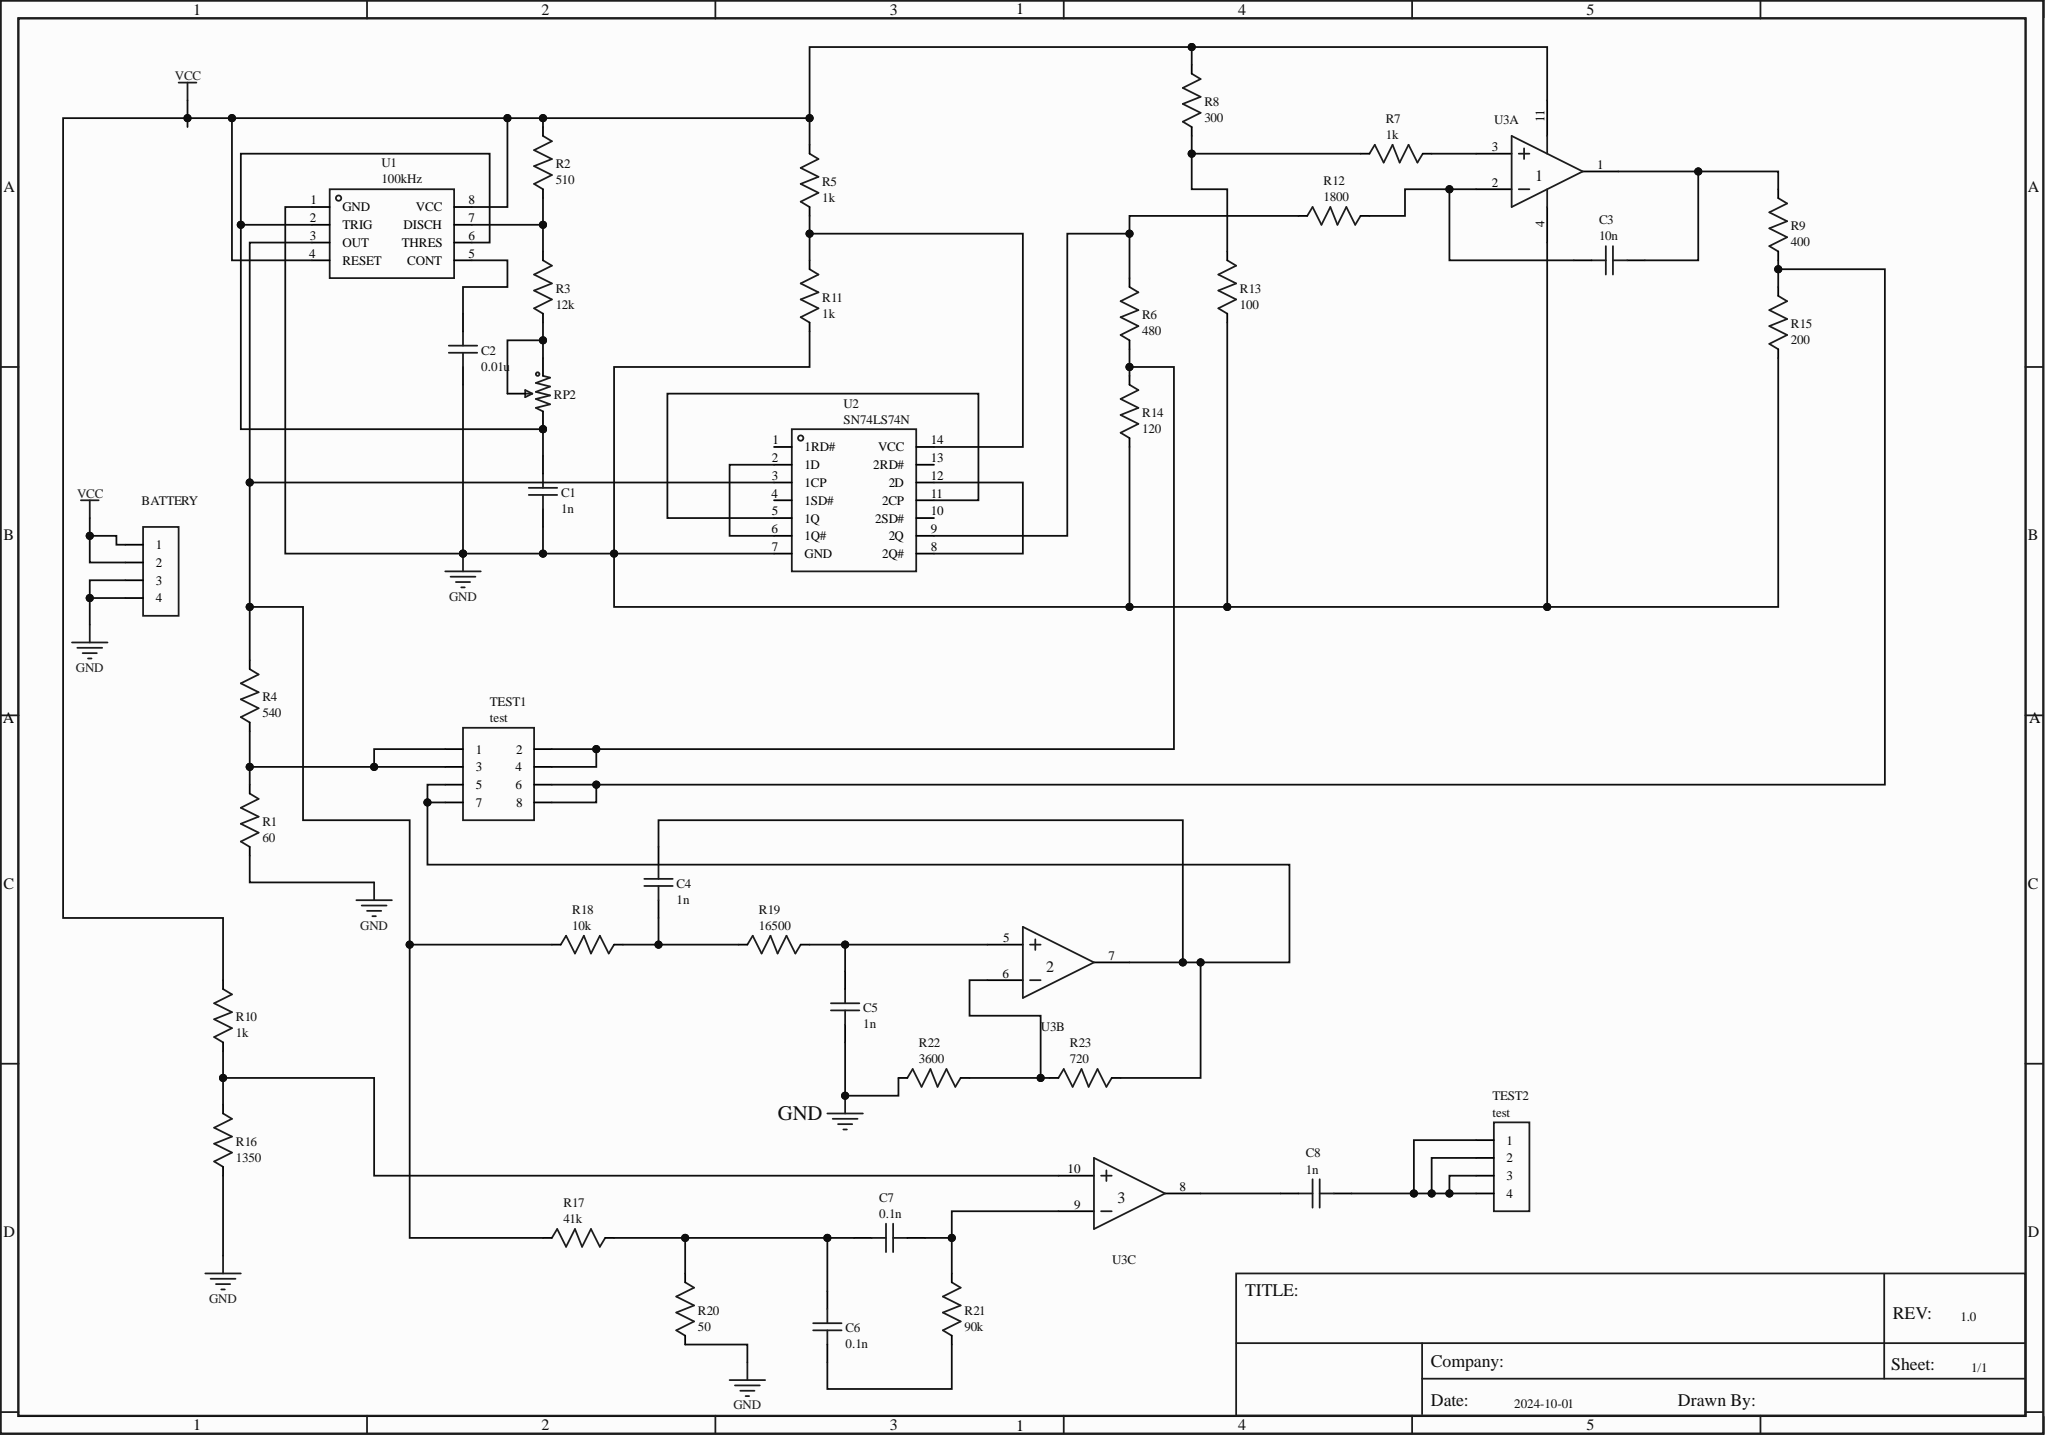Circuit board | Altium Designer | 38 parts | 29 nets
Bill of materials:
Comment,Description,Designator,Footprint,LibRef,Quantity
"HDR-M-2.54_1x4","","BATTERY","HDR-M-2.54_1X4","HDR-M-2.54_1x4","1"
"1n","","C1, C4, C5, C8","RAD-0.1","1n","4"
"0.01u","","C2","RAD-0.1","0.01u","1"
"10n","","C3","RAD-0.1","10n","1"
"0.1n","","C6, C7","RAD-0.1","0.1n","2"
"60","","R1","R_AXIAL-0.3","60","1"
"510","","R2","R_AXIAL-0.3","510","1"
"12k","","R3","R_AXIAL-0.3","12k","1"
"540","","R4","R_AXIAL-0.3","540","1"
"1k","","R5, R7, R10, R11","R_AXIAL-0.3","1k","4"
"480","","R6","R_AXIAL-0.3","480","1"
"300","","R8","R_AXIAL-0.3","300","1"
"400","","R9","R_AXIAL-0.3","400","1"
"1800","","R12","R_AXIAL-0.3","1800","1"
"100","","R13","R_AXIAL-0.3","100","1"
"120","","R14","R_AXIAL-0.3","120","1"
"200","","R15","R_AXIAL-0.3","200","1"
"1350","","R16","R_AXIAL-0.3","1350","1"
"41k","","R17","R_AXIAL-0.3","41k","1"
"10k","","R18","R_AXIAL-0.3","10k","1"
"16500","","R19","R_AXIAL-0.3","16500","1"
"50","","R20","R_AXIAL-0.3","50","1"
"90k","","R21","R_AXIAL-0.3","90k","1"
"3600","","R22","R_AXIAL-0.3","3600","1"
"720","","R23","R_AXIAL-0.3","720","1"
"R_3296W_US","","RP2","RES-ADJ-TH_3296W","R_3296W_US","1"
"test","","TEST1","HDR-M-2.54_2X4","test","1"
"test","","TEST2","HDR-M-2.54_1X4","test","1"
"100kHz","","U1","DIP-8_L9.8-W6.6-P2.54-LS7.6-BL","100kHz","1"
"SN74LS74N","","U2","DIP-14_L19.1-W6.4-P2.54-LS7.6-BL","SN74LS74N","1"
"LM324_C5157701","","U3","DIP-14_L18.9-W6.4-P2.54-LS7.6-BL","LM324_C5157701","1"
Netlist (Protel format):
[
BATTERY
HDR-M-2.54_1X4
HDR-M-2.54_1x4



]
[
C1
RAD-0.1
1n



]
[
C2
RAD-0.1
0.01u



]
[
C3
RAD-0.1
10n



]
[
C4
RAD-0.1
1n



]
[
C5
RAD-0.1
1n



]
[
C6
RAD-0.1
0.1n



]
[
C7
RAD-0.1
0.1n



]
[
C8
RAD-0.1
1n



]
[
R1
R_AXIAL-0.3
60



]
[
R2
R_AXIAL-0.3
510



]
[
R3
R_AXIAL-0.3
12k



]
[
R4
R_AXIAL-0.3
540



]
[
R5
R_AXIAL-0.3
1k



]
[
R6
R_AXIAL-0.3
480



]
[
R7
R_AXIAL-0.3
1k



]
[
R8
R_AXIAL-0.3
300



]
[
R9
R_AXIAL-0.3
400



]
[
R10
R_AXIAL-0.3
1k



]
[
R11
R_AXIAL-0.3
1k



]
[
R12
R_AXIAL-0.3
1800



]
[
R13
R_AXIAL-0.3
100



]
[
R14
R_AXIAL-0.3
120



]
[
R15
R_AXIAL-0.3
200



]
[
R16
R_AXIAL-0.3
1350



]
[
R17
R_AXIAL-0.3
41k



]
[
R18
R_AXIAL-0.3
10k



]
[
R19
R_AXIAL-0.3
16500



]
[
R20
R_AXIAL-0.3
50



]
[
R21
R_AXIAL-0.3
90k



]
[
R22
R_AXIAL-0.3
3600



]
[
R23
R_AXIAL-0.3
720



]
[
RP2
RES-ADJ-TH_3296W
R_3296W_US



]
[
TEST1
HDR-M-2.54_2X4
test



]
[
TEST2
HDR-M-2.54_1X4
test



]
[
U1
DIP-8_L9.8-W6.6-P2.54-LS7.6-BL
100kHz



]
[
U2
DIP-14_L19.1-W6.4-P2.54-LS7.6-BL
SN74LS74N



]
[
U3
DIP-14_L18.9-W6.4-P2.54-LS7.6-BL
LM324_C5157701



]
(
VCC
BATTERY-1
BATTERY-2
R2-2
R5-2
R8-2
R10-2
U1-4
U1-8
U3-11
)
(
NetU2_8
U2-8
U2-12
)
(
NetU2_5
U2-5
U2-11
)
(
NetU2_2
U2-2
U2-6
)
(
NetR22_1
R22-1
R23-2
U3-6
)
(
NetR10_1
R10-1
R16-2
U3-10
)
(
NetR9_2
R9-2
R15-1
TEST1-6
TEST1-8
)
(
NetR7_2
R7-2
R8-1
R13-2
)
(
NetR7_1
R7-1
U3-3
)
(
NetR6_2
R6-2
R12-2
U2-9
)
(
NetR6_1
R6-1
R14-2
TEST1-2
TEST1-4
)
(
NetR5_1
R5-1
R11-2
U2-14
)
(
NetR4_2
R4-2
R17-2
R18-2
U1-3
U2-3
)
(
NetR3_1
R3-1
RP2-1
RP2-2
)
(
NetR2_1
R2-1
R3-2
U1-7
)
(
NetR1_2
R1-2
R4-1
TEST1-1
TEST1-3
)
(
NetC8_2
C8-2
U3-8
)
(
NetC8_1
C8-1
TEST2-1
TEST2-2
TEST2-3
TEST2-4
)
(
NetC7_2
C7-2
R21-1
U3-9
)
(
NetC6_2
C6-2
R21-2
)
(
NetC6_1
C6-1
C7-1
R17-1
R20-1
)
(
NetC5_2
C5-2
R19-1
U3-5
)
(
NetC4_2
C4-2
R23-1
TEST1-5
TEST1-7
U3-7
)
(
NetC4_1
C4-1
R18-1
R19-2
)
(
NetC3_2
C3-2
R12-1
U3-2
)
(
NetC3_1
C3-1
R9-1
U3-1
)
(
NetC2_2
C2-2
U1-5
)
(
NetC1_2
C1-2
RP2-3
U1-2
U1-6
)
(
GND
BATTERY-3
BATTERY-4
C1-1
C2-1
C5-1
R1-1
R11-1
R13-1
R14-1
R15-2
R16-1
R20-2
R22-2
U1-1
U2-7
U3-4
)